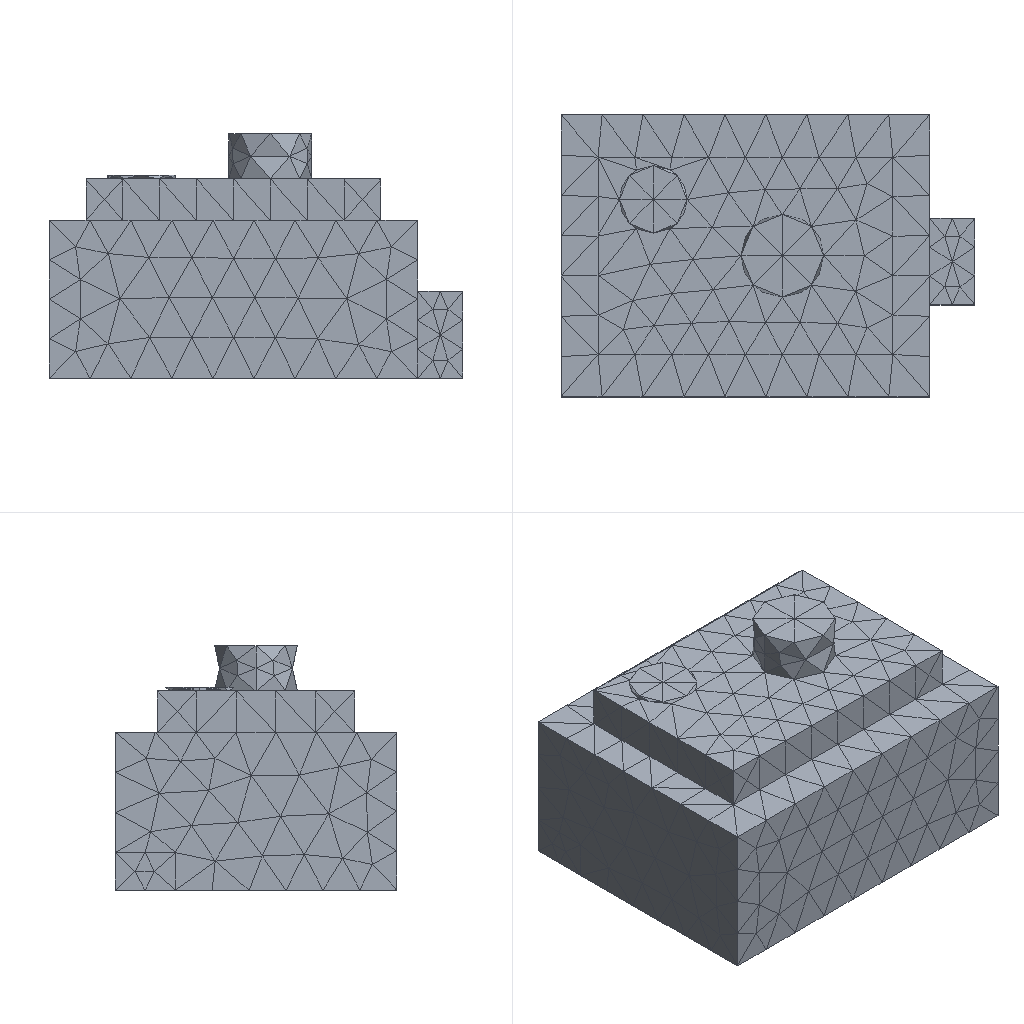Simulation study | ansys mapdl
Set-up summary:
category,name,step,type,value,unit,region
solver,ansys_mapdl
units,mm-N-s-tonne (MPa),,inferred,E=210000 density=
analysis,model,,static
mesh,nodes,,,4885
mesh,elements,,,2953
element_type,SOLID187,,,2953
material,mat 1,,E,210000
material,mat 1,,nu,0.3
load,,model,body load temp,,,all
load,,model,force,"1000 [dir=(0, 0, -1) n=193]",,node list
bc,,model,fixed,"[dofs=UX,UY,UZ n=5459]",,node list
Ansys APDL input file, long lists of numbers shortened:
/COM,ANSYS RELEASE 2026 R1           BUILD 26.1      UP20260202       09:08:46
/PREP7
/NOPR
/TITLE,2
ANTYPE, 0
*IF,_CDRDOFF,EQ,1,THEN     !if solid model was read in
_CDRDOFF=             !reset flag, numoffs already performed
*ELSE              !offset database for the following FE model
NUMOFF,NODE,     4885
NUMOFF,ELEM,     2953
NUMOFF,MAT ,        1
NUMOFF,TYPE,        1
*ENDIF
*SET,_RETURN ,  0.
*SET,_STATUS ,  0.
*SET,_UIQR   ,  193.
*SET,__FLOATPARAMETER__,  4885.
DOF,DELETE
ETBLOCK,        1,        1
(2i9,19a9)
        1      187        0        0        0        0        0        0        0        0        0        0        0        0        0        0        0        0        0        0        0
       -1
NBLOCK,6,SOLID,      4885,      4885
(3i9,6e21.13e3)
        1        0        0-3.3025000000000E+001 3.7500000000000E+001 1.0000000000000E+001
! (4884 more lines like these left out)
N,UNBL,LOC,       -1,
EBLOCK,19,SOLID,      2953,      2953
(19i10)
         1         1         1         1         0         0         0         0        10         0         1      1799      1800       457       478      2090      2091      2092      2093
! (5905 more lines like these left out)
        -1
MPTEMP,UNBL, 1, 1,  0.    ,
MPDATA,UNBL, 1,EX  ,       1, 1,  210000.000    ,
MPTEMP,UNBL, 1, 1,  0.    ,
MPDATA,UNBL, 1,NUXY,       1, 1, 0.3    ,
MPTEMP,UNBL, 1, 1,  0.    ,
MPDATA,UNBL, 1,PRXY,       1, 1, 0.3    ,
EXTOPT,ATTR,      0,      0,      0
EXTOPT,ESIZE,  0,  0.
EXTOPT,ACLEAR,      0
TREF,  0.
IRLF,  0
BFUNIF,TEMP,_TINY
ACEL,  0.    ,  0.    ,  0.
OMEGA,  0.    ,  0.    ,  0.
DOMEGA,  0.    ,  0.    ,  0.
CGLOC,  0.    ,  0.    ,  0.
CGOMEGA,  0.    ,  0.    ,  0.
DCGOMG,  0.    ,  0.    ,  0.
KUSE,     0
TIME,  0.
ALPHAD,  0.
BETAD,  0.
DMPRAT,  0.
DMPSTR,  0.
CRPLIM, 0.1    ,   0
CRPLIM,  0.    ,   1
NCNV,     0, 1.000000000E+12,     0,  0.    ,  0.
NEQIT,     0
ERESX,DEFA
DBLOCK,      5459
(i9,a6,2(pg16.9))
        1  UX    0.00000000      0.00000000
! (5458 more lines like these left out)
       -1
FBLOCK,       193
(i9,a6,2(pg16.9))
      792  FZ   -5.18134715      0.00000000
! (192 more lines like these left out)
       -1
/GO
FINISH
Results summary:
result,analysis_type_db,,,static,unstated
result,n_sets,,,1,unstated
result,load_steps[0].set,load_step=1,,1,unstated
result,load_steps[0].substep,load_step=1,,1,unstated
result,load_steps[0].time,load_step=1,,1,unstated
result,load_steps[0].freq,load_step=1,,1,unstated
result,load_steps[0].max_usum,load_step=1,,0.0002334,unstated
result,load_steps[0].max_seqv,load_step=1,,14.497,unstated
result,load_steps[0].reaction_sum.FX,load_step=1,,-1.14238e-11,unstated
result,load_steps[0].reaction_sum.FY,load_step=1,,-1.43174e-11,unstated
result,load_steps[0].reaction_sum.FZ,load_step=1,,1000,unstated
result,load_steps[0].reaction_sum.MX,load_step=1,,0,unstated
result,load_steps[0].reaction_sum.MY,load_step=1,,0,unstated
result,load_steps[0].reaction_sum.MZ,load_step=1,,0,unstated
result,convergence,,,results present for all listed sets,unstated